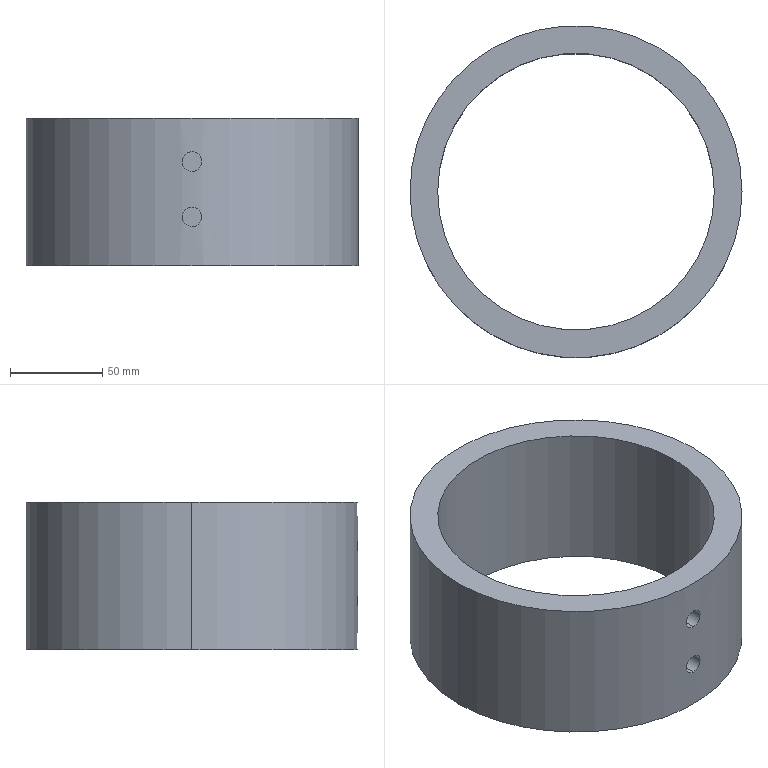Part | SolidWorks | features BaseBody 1 | 1 solid | 10 faces | box 180 x 180 x 80 mm | volume 619388 mm3 | cylinder 8 | plane 2 | commonest cylinder face diameters 10.6 x4 150 x2 180 x2
STEP:
#1=CARTESIAN_POINT('',(0.,-295.,82.3));
#2=VERTEX_POINT('',#1);
#3=CARTESIAN_POINT('',(0.,-295.,71.7));
#4=VERTEX_POINT('',#3);
#5=CARTESIAN_POINT('',(0.,-295.,82.3));
#6=CARTESIAN_POINT('',(-0.3503,-295.,82.3));
#7=CARTESIAN_POINT('',(-0.6947,-294.998,82.266));
#8=CARTESIAN_POINT('',(-1.203,-294.992,82.165));
#9=CARTESIAN_POINT('',(-1.371,-294.99,82.123));
#10=CARTESIAN_POINT('',(-1.704,-294.984,82.022));
#11=CARTESIAN_POINT('',(-1.869,-294.981,81.962));
#12=CARTESIAN_POINT('',(-2.351,-294.97,81.763));
#13=CARTESIAN_POINT('',(-2.655,-294.961,81.6));
#14=CARTESIAN_POINT('',(-3.231,-294.942,81.215));
#15=CARTESIAN_POINT('',(-3.504,-294.932,80.991));
#16=CARTESIAN_POINT('',(-3.993,-294.912,80.502));
#17=CARTESIAN_POINT('',(-4.212,-294.902,80.236));
#18=CARTESIAN_POINT('',(-4.6,-294.883,79.656));
#19=CARTESIAN_POINT('',(-4.764,-294.874,79.348));
#20=CARTESIAN_POINT('',(-5.028,-294.86,78.71));
#21=CARTESIAN_POINT('',(-5.13,-294.854,78.376));
#22=CARTESIAN_POINT('',(-5.266,-294.846,77.692));
#23=CARTESIAN_POINT('',(-5.3,-294.844,77.348));
#24=CARTESIAN_POINT('',(-5.3,-294.844,76.656));
#25=CARTESIAN_POINT('',(-5.266,-294.846,76.305));
#26=CARTESIAN_POINT('',(-5.13,-294.854,75.625));
#27=CARTESIAN_POINT('',(-5.03,-294.859,75.295));
#28=CARTESIAN_POINT('',(-4.831,-294.87,74.813));
#29=CARTESIAN_POINT('',(-4.756,-294.874,74.654));
#30=CARTESIAN_POINT('',(-4.592,-294.883,74.347));
#31=CARTESIAN_POINT('',(-4.503,-294.887,74.199));
#32=CARTESIAN_POINT('',(-4.215,-294.901,73.768));
#33=CARTESIAN_POINT('',(-3.996,-294.912,73.501));
#34=CARTESIAN_POINT('',(-3.501,-294.932,73.006));
#35=CARTESIAN_POINT('',(-3.233,-294.942,72.786));
#36=CARTESIAN_POINT('',(-2.803,-294.956,72.498));
#37=CARTESIAN_POINT('',(-2.654,-294.961,72.409));
#38=CARTESIAN_POINT('',(-2.348,-294.97,72.245));
#39=CARTESIAN_POINT('',(-2.189,-294.974,72.17));
#40=CARTESIAN_POINT('',(-1.707,-294.984,71.97));
#41=CARTESIAN_POINT('',(-1.377,-294.99,71.87));
#42=CARTESIAN_POINT('',(-0.6973,-294.998,71.735));
#43=CARTESIAN_POINT('',(-0.3459,-295.,71.7));
#44=CARTESIAN_POINT('',(0.,-295.,71.7));
#45=B_SPLINE_CURVE_WITH_KNOTS('',3,(#5,#6,#7,#8,#9,#10,#11,#12,#13,#14,#15,#16,#17,#18,#19,#20,#21,#22,#23,#24,#25,#26,#27,#28,#29,#30,#31,#32,#33,#34,#35,#36,#37,#38,#39,#40,#41,#42,#43,#44),.UNSPECIFIED.,.F.,.F.,(4,2,2,2,2,2,2,2,2,2,2,2,2,2,2,2,2,2,2,4),(0.,0.001036,0.001554,0.002072,0.003108,0.004143,0.005179,0.006215,0.007251,0.008287,0.009323,0.01036,0.01088,0.01139,0.01243,0.01347,0.01398,0.0145,0.01554,0.01657),.UNSPECIFIED.);
#46=EDGE_CURVE('',#2,#4,#45,.T.);
#47=ORIENTED_EDGE('',*,*,#46,.T.);
#48=CARTESIAN_POINT('',(0.,-280.,71.7));
#49=VERTEX_POINT('',#48);
#50=CARTESIAN_POINT('',(0.,-402.5,71.7));
#51=DIRECTION('',(0.,1.,0.));
#52=VECTOR('',#51,1000.);
#53=LINE('',#50,#52);
#54=EDGE_CURVE('',#4,#49,#53,.T.);
#55=ORIENTED_EDGE('',*,*,#54,.T.);
#56=CARTESIAN_POINT('',(0.,-280.,82.3));
#57=VERTEX_POINT('',#56);
#58=CARTESIAN_POINT('',(0.,-280.,82.3));
#59=CARTESIAN_POINT('',(-0.3503,-280.,82.3));
#60=CARTESIAN_POINT('',(-0.6947,-279.998,82.266));
#61=CARTESIAN_POINT('',(-1.203,-279.991,82.165));
#62=CARTESIAN_POINT('',(-1.371,-279.988,82.123));
#63=CARTESIAN_POINT('',(-1.704,-279.981,82.022));
#64=CARTESIAN_POINT('',(-1.869,-279.977,81.962));
#65=CARTESIAN_POINT('',(-2.351,-279.964,81.763));
#66=CARTESIAN_POINT('',(-2.655,-279.954,81.6));
#67=CARTESIAN_POINT('',(-3.231,-279.931,81.215));
#68=CARTESIAN_POINT('',(-3.504,-279.919,80.991));
#69=CARTESIAN_POINT('',(-3.993,-279.894,80.503));
#70=CARTESIAN_POINT('',(-4.212,-279.882,80.236));
#71=CARTESIAN_POINT('',(-4.6,-279.859,79.656));
#72=CARTESIAN_POINT('',(-4.764,-279.849,79.348));
#73=CARTESIAN_POINT('',(-5.028,-279.831,78.71));
#74=CARTESIAN_POINT('',(-5.13,-279.824,78.376));
#75=CARTESIAN_POINT('',(-5.266,-279.815,77.692));
#76=CARTESIAN_POINT('',(-5.3,-279.813,77.348));
#77=CARTESIAN_POINT('',(-5.3,-279.812,76.656));
#78=CARTESIAN_POINT('',(-5.266,-279.815,76.305));
#79=CARTESIAN_POINT('',(-5.13,-279.824,75.625));
#80=CARTESIAN_POINT('',(-5.03,-279.831,75.295));
#81=CARTESIAN_POINT('',(-4.831,-279.844,74.813));
#82=CARTESIAN_POINT('',(-4.756,-279.849,74.654));
#83=CARTESIAN_POINT('',(-4.592,-279.859,74.347));
#84=CARTESIAN_POINT('',(-4.503,-279.865,74.199));
#85=CARTESIAN_POINT('',(-4.215,-279.882,73.768));
#86=CARTESIAN_POINT('',(-3.996,-279.894,73.501));
#87=CARTESIAN_POINT('',(-3.501,-279.919,73.006));
#88=CARTESIAN_POINT('',(-3.233,-279.931,72.786));
#89=CARTESIAN_POINT('',(-2.803,-279.948,72.498));
#90=CARTESIAN_POINT('',(-2.654,-279.953,72.409));
#91=CARTESIAN_POINT('',(-2.348,-279.963,72.245));
#92=CARTESIAN_POINT('',(-2.189,-279.968,72.17));
#93=CARTESIAN_POINT('',(-1.707,-279.981,71.97));
#94=CARTESIAN_POINT('',(-1.377,-279.988,71.87));
#95=CARTESIAN_POINT('',(-0.6973,-279.998,71.735));
#96=CARTESIAN_POINT('',(-0.346,-280.,71.7));
#97=CARTESIAN_POINT('',(0.,-280.,71.7));
#98=B_SPLINE_CURVE_WITH_KNOTS('',3,(#58,#59,#60,#61,#62,#63,#64,#65,#66,#67,#68,#69,#70,#71,#72,#73,#74,#75,#76,#77,#78,#79,#80,#81,#82,#83,#84,#85,#86,#87,#88,#89,#90,#91,#92,#93,#94,#95,#96,#97),.UNSPECIFIED.,.F.,.F.,(4,2,2,2,2,2,2,2,2,2,2,2,2,2,2,2,2,2,2,4),(0.,0.001036,0.001554,0.002072,0.003108,0.004144,0.00518,0.006216,0.007252,0.008288,0.009324,0.01036,0.01088,0.0114,0.01243,0.01347,0.01399,0.0145,0.01554,0.01658),.UNSPECIFIED.);
#99=EDGE_CURVE('',#57,#49,#98,.T.);
#100=ORIENTED_EDGE('',*,*,#99,.F.);
#101=CARTESIAN_POINT('',(0.,-402.5,82.3));
#102=DIRECTION('',(0.,1.,0.));
#103=VECTOR('',#102,1000.);
#104=LINE('',#101,#103);
#105=EDGE_CURVE('',#2,#57,#104,.T.);
#106=ORIENTED_EDGE('',*,*,#105,.F.);
#107=EDGE_LOOP('',(#47,#55,#100,#106));
#108=FACE_OUTER_BOUND('',#107,.T.);
#109=CARTESIAN_POINT('',(0.,-402.5,77.));
#110=DIRECTION('',(0.,1.,0.));
#111=DIRECTION('',(0.,0.,1.));
#112=AXIS2_PLACEMENT_3D('',#109,#110,#111);
#113=CYLINDRICAL_SURFACE('',#112,5.3);
#114=ADVANCED_FACE('',(#108),#113,.F.);
#115=CARTESIAN_POINT('',(0.,-295.,112.3));
#116=VERTEX_POINT('',#115);
#117=CARTESIAN_POINT('',(0.,-295.,101.7));
#118=VERTEX_POINT('',#117);
#119=CARTESIAN_POINT('',(0.,-295.,112.3));
#120=CARTESIAN_POINT('',(-0.3503,-295.,112.3));
#121=CARTESIAN_POINT('',(-0.6947,-294.998,112.266));
#122=CARTESIAN_POINT('',(-1.203,-294.992,112.165));
#123=CARTESIAN_POINT('',(-1.371,-294.99,112.123));
#124=CARTESIAN_POINT('',(-1.704,-294.984,112.022));
#125=CARTESIAN_POINT('',(-1.869,-294.981,111.962));
#126=CARTESIAN_POINT('',(-2.351,-294.97,111.763));
#127=CARTESIAN_POINT('',(-2.655,-294.961,111.6));
#128=CARTESIAN_POINT('',(-3.231,-294.942,111.215));
#129=CARTESIAN_POINT('',(-3.504,-294.932,110.991));
#130=CARTESIAN_POINT('',(-3.993,-294.912,110.502));
#131=CARTESIAN_POINT('',(-4.212,-294.902,110.236));
#132=CARTESIAN_POINT('',(-4.6,-294.883,109.656));
#133=CARTESIAN_POINT('',(-4.764,-294.874,109.348));
#134=CARTESIAN_POINT('',(-5.028,-294.86,108.71));
#135=CARTESIAN_POINT('',(-5.13,-294.854,108.376));
#136=CARTESIAN_POINT('',(-5.266,-294.846,107.692));
#137=CARTESIAN_POINT('',(-5.3,-294.844,107.348));
#138=CARTESIAN_POINT('',(-5.3,-294.844,106.656));
#139=CARTESIAN_POINT('',(-5.266,-294.846,106.305));
#140=CARTESIAN_POINT('',(-5.13,-294.854,105.625));
#141=CARTESIAN_POINT('',(-5.03,-294.859,105.295));
#142=CARTESIAN_POINT('',(-4.831,-294.87,104.813));
#143=CARTESIAN_POINT('',(-4.756,-294.874,104.654));
#144=CARTESIAN_POINT('',(-4.592,-294.883,104.347));
#145=CARTESIAN_POINT('',(-4.503,-294.887,104.199));
#146=CARTESIAN_POINT('',(-4.215,-294.901,103.768));
#147=CARTESIAN_POINT('',(-3.996,-294.912,103.501));
#148=CARTESIAN_POINT('',(-3.501,-294.932,103.006));
#149=CARTESIAN_POINT('',(-3.233,-294.942,102.786));
#150=CARTESIAN_POINT('',(-2.803,-294.956,102.498));
#151=CARTESIAN_POINT('',(-2.654,-294.961,102.409));
#152=CARTESIAN_POINT('',(-2.348,-294.97,102.245));
#153=CARTESIAN_POINT('',(-2.189,-294.974,102.17));
#154=CARTESIAN_POINT('',(-1.707,-294.984,101.97));
#155=CARTESIAN_POINT('',(-1.377,-294.99,101.87));
#156=CARTESIAN_POINT('',(-0.6973,-294.998,101.735));
#157=CARTESIAN_POINT('',(-0.3459,-295.,101.7));
#158=CARTESIAN_POINT('',(0.,-295.,101.7));
#159=B_SPLINE_CURVE_WITH_KNOTS('',3,(#119,#120,#121,#122,#123,#124,#125,#126,#127,#128,#129,#130,#131,#132,#133,#134,#135,#136,#137,#138,#139,#140,#141,#142,#143,#144,#145,#146,#147,#148,#149,#150,#151,#152,#153,#154,#155,#156,#157,#158),.UNSPECIFIED.,.F.,.F.,(4,2,2,2,2,2,2,2,2,2,2,2,2,2,2,2,2,2,2,4),(0.,0.001036,0.001554,0.002072,0.003108,0.004143,0.005179,0.006215,0.007251,0.008287,0.009323,0.01036,0.01088,0.01139,0.01243,0.01347,0.01398,0.0145,0.01554,0.01657),.UNSPECIFIED.);
#160=EDGE_CURVE('',#116,#118,#159,.T.);
#161=ORIENTED_EDGE('',*,*,#160,.T.);
#162=CARTESIAN_POINT('',(0.,-280.,101.7));
#163=VERTEX_POINT('',#162);
#164=CARTESIAN_POINT('',(0.,-403.,101.7));
#165=DIRECTION('',(0.,1.,0.));
#166=VECTOR('',#165,1000.);
#167=LINE('',#164,#166);
#168=EDGE_CURVE('',#118,#163,#167,.T.);
#169=ORIENTED_EDGE('',*,*,#168,.T.);
#170=CARTESIAN_POINT('',(0.,-280.,112.3));
#171=VERTEX_POINT('',#170);
#172=CARTESIAN_POINT('',(0.,-280.,112.3));
#173=CARTESIAN_POINT('',(-0.3503,-280.,112.3));
#174=CARTESIAN_POINT('',(-0.6947,-279.998,112.266));
#175=CARTESIAN_POINT('',(-1.203,-279.991,112.165));
#176=CARTESIAN_POINT('',(-1.371,-279.988,112.123));
#177=CARTESIAN_POINT('',(-1.704,-279.981,112.022));
#178=CARTESIAN_POINT('',(-1.869,-279.977,111.962));
#179=CARTESIAN_POINT('',(-2.351,-279.964,111.763));
#180=CARTESIAN_POINT('',(-2.655,-279.954,111.6));
#181=CARTESIAN_POINT('',(-3.231,-279.931,111.215));
#182=CARTESIAN_POINT('',(-3.504,-279.919,110.991));
#183=CARTESIAN_POINT('',(-3.993,-279.894,110.503));
#184=CARTESIAN_POINT('',(-4.212,-279.882,110.236));
#185=CARTESIAN_POINT('',(-4.6,-279.859,109.656));
#186=CARTESIAN_POINT('',(-4.764,-279.849,109.348));
#187=CARTESIAN_POINT('',(-5.028,-279.831,108.71));
#188=CARTESIAN_POINT('',(-5.13,-279.824,108.376));
#189=CARTESIAN_POINT('',(-5.266,-279.815,107.692));
#190=CARTESIAN_POINT('',(-5.3,-279.813,107.348));
#191=CARTESIAN_POINT('',(-5.3,-279.812,106.656));
#192=CARTESIAN_POINT('',(-5.266,-279.815,106.305));
#193=CARTESIAN_POINT('',(-5.13,-279.824,105.625));
#194=CARTESIAN_POINT('',(-5.03,-279.831,105.295));
#195=CARTESIAN_POINT('',(-4.831,-279.844,104.813));
#196=CARTESIAN_POINT('',(-4.756,-279.849,104.654));
#197=CARTESIAN_POINT('',(-4.592,-279.859,104.347));
#198=CARTESIAN_POINT('',(-4.503,-279.865,104.199));
#199=CARTESIAN_POINT('',(-4.215,-279.882,103.768));
#200=CARTESIAN_POINT('',(-3.996,-279.894,103.501));
#201=CARTESIAN_POINT('',(-3.501,-279.919,103.006));
#202=CARTESIAN_POINT('',(-3.233,-279.931,102.786));
#203=CARTESIAN_POINT('',(-2.803,-279.948,102.498));
#204=CARTESIAN_POINT('',(-2.654,-279.953,102.409));
#205=CARTESIAN_POINT('',(-2.348,-279.963,102.245));
#206=CARTESIAN_POINT('',(-2.189,-279.968,102.17));
#207=CARTESIAN_POINT('',(-1.707,-279.981,101.97));
#208=CARTESIAN_POINT('',(-1.377,-279.988,101.87));
#209=CARTESIAN_POINT('',(-0.6973,-279.998,101.735));
#210=CARTESIAN_POINT('',(-0.346,-280.,101.7));
#211=CARTESIAN_POINT('',(0.,-280.,101.7));
#212=B_SPLINE_CURVE_WITH_KNOTS('',3,(#172,#173,#174,#175,#176,#177,#178,#179,#180,#181,#182,#183,#184,#185,#186,#187,#188,#189,#190,#191,#192,#193,#194,#195,#196,#197,#198,#199,#200,#201,#202,#203,#204,#205,#206,#207,#208,#209,#210,#211),.UNSPECIFIED.,.F.,.F.,(4,2,2,2,2,2,2,2,2,2,2,2,2,2,2,2,2,2,2,4),(0.,0.001036,0.001554,0.002072,0.003108,0.004144,0.00518,0.006216,0.007252,0.008288,0.009324,0.01036,0.01088,0.0114,0.01243,0.01347,0.01399,0.0145,0.01554,0.01658),.UNSPECIFIED.);
#213=EDGE_CURVE('',#171,#163,#212,.T.);
#214=ORIENTED_EDGE('',*,*,#213,.F.);
#215=CARTESIAN_POINT('',(0.,-403.,112.3));
#216=DIRECTION('',(0.,1.,0.));
#217=VECTOR('',#216,1000.);
#218=LINE('',#215,#217);
#219=EDGE_CURVE('',#116,#171,#218,.T.);
#220=ORIENTED_EDGE('',*,*,#219,.F.);
#221=EDGE_LOOP('',(#161,#169,#214,#220));
#222=FACE_OUTER_BOUND('',#221,.T.);
#223=CARTESIAN_POINT('',(0.,-403.,107.));
#224=DIRECTION('',(0.,1.,0.));
#225=DIRECTION('',(0.,0.,1.));
#226=AXIS2_PLACEMENT_3D('',#223,#224,#225);
#227=CYLINDRICAL_SURFACE('',#226,5.3);
#228=ADVANCED_FACE('',(#222),#227,.F.);
#229=ORIENTED_EDGE('',*,*,#99,.T.);
#230=CARTESIAN_POINT('',(0.,-280.,71.7));
#231=CARTESIAN_POINT('',(0.3459,-280.,71.7));
#232=CARTESIAN_POINT('',(0.6897,-279.998,71.734));
#233=CARTESIAN_POINT('',(1.202,-279.991,71.835));
#234=CARTESIAN_POINT('',(1.373,-279.988,71.878));
#235=CARTESIAN_POINT('',(1.705,-279.981,71.979));
#236=CARTESIAN_POINT('',(1.867,-279.977,72.037));
#237=CARTESIAN_POINT('',(2.346,-279.964,72.235));
#238=CARTESIAN_POINT('',(2.654,-279.954,72.399));
#239=CARTESIAN_POINT('',(3.234,-279.931,72.786));
#240=CARTESIAN_POINT('',(3.501,-279.919,73.006));
#241=CARTESIAN_POINT('',(3.99,-279.894,73.494));
#242=CARTESIAN_POINT('',(4.213,-279.882,73.766));
#243=CARTESIAN_POINT('',(4.599,-279.859,74.342));
#244=CARTESIAN_POINT('',(4.761,-279.849,74.646));
#245=CARTESIAN_POINT('',(4.961,-279.836,75.127));
#246=CARTESIAN_POINT('',(5.02,-279.832,75.293));
#247=CARTESIAN_POINT('',(5.122,-279.825,75.626));
#248=CARTESIAN_POINT('',(5.164,-279.822,75.794));
#249=CARTESIAN_POINT('',(5.265,-279.815,76.302));
#250=CARTESIAN_POINT('',(5.3,-279.813,76.646));
#251=CARTESIAN_POINT('',(5.3,-279.812,77.346));
#252=CARTESIAN_POINT('',(5.266,-279.815,77.691));
#253=CARTESIAN_POINT('',(5.165,-279.822,78.199));
#254=CARTESIAN_POINT('',(5.124,-279.825,78.367));
#255=CARTESIAN_POINT('',(5.023,-279.832,78.7));
#256=CARTESIAN_POINT('',(4.964,-279.836,78.865));
#257=CARTESIAN_POINT('',(4.765,-279.849,79.347));
#258=CARTESIAN_POINT('',(4.602,-279.859,79.652));
#259=CARTESIAN_POINT('',(4.218,-279.882,80.227));
#260=CARTESIAN_POINT('',(3.995,-279.894,80.5));
#261=CARTESIAN_POINT('',(3.506,-279.918,80.99));
#262=CARTESIAN_POINT('',(3.24,-279.931,81.209));
#263=CARTESIAN_POINT('',(2.806,-279.948,81.5));
#264=CARTESIAN_POINT('',(2.655,-279.953,81.59));
#265=CARTESIAN_POINT('',(2.349,-279.963,81.754));
#266=CARTESIAN_POINT('',(2.193,-279.968,81.828));
#267=CARTESIAN_POINT('',(1.715,-279.981,82.027));
#268=CARTESIAN_POINT('',(1.382,-279.988,82.129));
#269=CARTESIAN_POINT('',(0.6967,-279.998,82.266));
#270=CARTESIAN_POINT('',(0.3502,-280.,82.3));
#271=CARTESIAN_POINT('',(0.,-280.,82.3));
#272=B_SPLINE_CURVE_WITH_KNOTS('',3,(#230,#231,#232,#233,#234,#235,#236,#237,#238,#239,#240,#241,#242,#243,#244,#245,#246,#247,#248,#249,#250,#251,#252,#253,#254,#255,#256,#257,#258,#259,#260,#261,#262,#263,#264,#265,#266,#267,#268,#269,#270,#271),.UNSPECIFIED.,.F.,.F.,(4,2,2,2,2,2,2,2,2,2,2,2,2,2,2,2,2,2,2,2,4),(0.01658,0.01761,0.01813,0.01865,0.01968,0.02072,0.02175,0.02279,0.02331,0.02383,0.02486,0.0259,0.02641,0.02693,0.02797,0.029,0.03004,0.03056,0.03108,0.03211,0.03315),.UNSPECIFIED.);
#273=EDGE_CURVE('',#49,#57,#272,.T.);
#274=ORIENTED_EDGE('',*,*,#273,.T.);
#275=EDGE_LOOP('',(#229,#274));
#276=FACE_BOUND('',#275,.T.);
#277=ORIENTED_EDGE('',*,*,#213,.T.);
#278=CARTESIAN_POINT('',(0.,-280.,101.7));
#279=CARTESIAN_POINT('',(0.3459,-280.,101.7));
#280=CARTESIAN_POINT('',(0.6897,-279.998,101.734));
#281=CARTESIAN_POINT('',(1.202,-279.991,101.835));
#282=CARTESIAN_POINT('',(1.373,-279.988,101.878));
#283=CARTESIAN_POINT('',(1.705,-279.981,101.979));
#284=CARTESIAN_POINT('',(1.867,-279.977,102.037));
#285=CARTESIAN_POINT('',(2.346,-279.964,102.235));
#286=CARTESIAN_POINT('',(2.654,-279.954,102.399));
#287=CARTESIAN_POINT('',(3.234,-279.931,102.786));
#288=CARTESIAN_POINT('',(3.501,-279.919,103.006));
#289=CARTESIAN_POINT('',(3.99,-279.894,103.494));
#290=CARTESIAN_POINT('',(4.213,-279.882,103.766));
#291=CARTESIAN_POINT('',(4.599,-279.859,104.342));
#292=CARTESIAN_POINT('',(4.761,-279.849,104.646));
#293=CARTESIAN_POINT('',(4.961,-279.836,105.127));
#294=CARTESIAN_POINT('',(5.02,-279.832,105.293));
#295=CARTESIAN_POINT('',(5.122,-279.825,105.626));
#296=CARTESIAN_POINT('',(5.164,-279.822,105.794));
#297=CARTESIAN_POINT('',(5.265,-279.815,106.302));
#298=CARTESIAN_POINT('',(5.3,-279.813,106.646));
#299=CARTESIAN_POINT('',(5.3,-279.812,107.346));
#300=CARTESIAN_POINT('',(5.266,-279.815,107.691));
#301=CARTESIAN_POINT('',(5.165,-279.822,108.199));
#302=CARTESIAN_POINT('',(5.124,-279.825,108.367));
#303=CARTESIAN_POINT('',(5.023,-279.832,108.7));
#304=CARTESIAN_POINT('',(4.964,-279.836,108.865));
#305=CARTESIAN_POINT('',(4.765,-279.849,109.347));
#306=CARTESIAN_POINT('',(4.602,-279.859,109.652));
#307=CARTESIAN_POINT('',(4.218,-279.882,110.227));
#308=CARTESIAN_POINT('',(3.995,-279.894,110.5));
#309=CARTESIAN_POINT('',(3.506,-279.918,110.99));
#310=CARTESIAN_POINT('',(3.24,-279.931,111.209));
#311=CARTESIAN_POINT('',(2.806,-279.948,111.5));
#312=CARTESIAN_POINT('',(2.655,-279.953,111.59));
#313=CARTESIAN_POINT('',(2.349,-279.963,111.754));
#314=CARTESIAN_POINT('',(2.193,-279.968,111.828));
#315=CARTESIAN_POINT('',(1.715,-279.981,112.027));
#316=CARTESIAN_POINT('',(1.382,-279.988,112.129));
#317=CARTESIAN_POINT('',(0.6967,-279.998,112.266));
#318=CARTESIAN_POINT('',(0.3502,-280.,112.3));
#319=CARTESIAN_POINT('',(0.,-280.,112.3));
#320=B_SPLINE_CURVE_WITH_KNOTS('',3,(#278,#279,#280,#281,#282,#283,#284,#285,#286,#287,#288,#289,#290,#291,#292,#293,#294,#295,#296,#297,#298,#299,#300,#301,#302,#303,#304,#305,#306,#307,#308,#309,#310,#311,#312,#313,#314,#315,#316,#317,#318,#319),.UNSPECIFIED.,.F.,.F.,(4,2,2,2,2,2,2,2,2,2,2,2,2,2,2,2,2,2,2,2,4),(0.01658,0.01761,0.01813,0.01865,0.01968,0.02072,0.02175,0.02279,0.02331,0.02383,0.02486,0.0259,0.02641,0.02693,0.02797,0.029,0.03004,0.03056,0.03108,0.03211,0.03315),.UNSPECIFIED.);
#321=EDGE_CURVE('',#163,#171,#320,.T.);
#322=ORIENTED_EDGE('',*,*,#321,.T.);
#323=EDGE_LOOP('',(#277,#322));
#324=FACE_BOUND('',#323,.T.);
#325=CARTESIAN_POINT('',(-75.,-205.,130.5));
#326=VERTEX_POINT('',#325);
#327=CARTESIAN_POINT('',(75.,-205.,130.5));
#328=VERTEX_POINT('',#327);
#329=CARTESIAN_POINT('',(0.,-205.,130.5));
#330=DIRECTION('',(0.,0.,1.));
#331=DIRECTION('',(1.,0.,0.));
#332=AXIS2_PLACEMENT_3D('',#329,#330,#331);
#333=CIRCLE('',#332,75.);
#334=EDGE_CURVE('',#326,#328,#333,.T.);
#335=ORIENTED_EDGE('',*,*,#334,.T.);
#336=CARTESIAN_POINT('',(75.,-205.,50.5));
#337=VERTEX_POINT('',#336);
#338=CARTESIAN_POINT('',(75.,-205.,170.5));
#339=DIRECTION('',(0.,0.,-1.));
#340=VECTOR('',#339,1000.);
#341=LINE('',#338,#340);
#342=EDGE_CURVE('',#328,#337,#341,.T.);
#343=ORIENTED_EDGE('',*,*,#342,.T.);
#344=CARTESIAN_POINT('',(-75.,-205.,50.5));
#345=VERTEX_POINT('',#344);
#346=CARTESIAN_POINT('',(0.,-205.,50.5));
#347=DIRECTION('',(0.,0.,-1.));
#348=DIRECTION('',(-1.,0.,0.));
#349=AXIS2_PLACEMENT_3D('',#346,#347,#348);
#350=CIRCLE('',#349,75.);
#351=EDGE_CURVE('',#337,#345,#350,.T.);
#352=ORIENTED_EDGE('',*,*,#351,.T.);
#353=CARTESIAN_POINT('',(-75.,-205.,170.5));
#354=DIRECTION('',(0.,0.,-1.));
#355=VECTOR('',#354,1000.);
#356=LINE('',#353,#355);
#357=EDGE_CURVE('',#326,#345,#356,.T.);
#358=ORIENTED_EDGE('',*,*,#357,.F.);
#359=EDGE_LOOP('',(#335,#343,#352,#358));
#360=FACE_OUTER_BOUND('',#359,.T.);
#361=CARTESIAN_POINT('',(0.,-205.,170.5));
#362=DIRECTION('',(0.,0.,-1.));
#363=DIRECTION('',(-1.,0.,0.));
#364=AXIS2_PLACEMENT_3D('',#361,#362,#363);
#365=CYLINDRICAL_SURFACE('',#364,75.);
#366=ADVANCED_FACE('',(#276,#324,#360),#365,.F.);
#367=CARTESIAN_POINT('',(-90.,-205.,130.5));
#368=VERTEX_POINT('',#367);
#369=CARTESIAN_POINT('',(90.,-205.,130.5));
#370=VERTEX_POINT('',#369);
#371=CARTESIAN_POINT('',(0.,-205.,130.5));
#372=DIRECTION('',(0.,0.,-1.));
#373=DIRECTION('',(-1.,0.,0.));
#374=AXIS2_PLACEMENT_3D('',#371,#372,#373);
#375=CIRCLE('',#374,90.);
#376=EDGE_CURVE('',#368,#370,#375,.T.);
#377=ORIENTED_EDGE('',*,*,#376,.T.);
#378=CARTESIAN_POINT('',(90.,-205.,50.5));
#379=VERTEX_POINT('',#378);
#380=CARTESIAN_POINT('',(90.,-205.,130.5));
#381=DIRECTION('',(0.,0.,-1.));
#382=VECTOR('',#381,1000.);
#383=LINE('',#380,#382);
#384=EDGE_CURVE('',#370,#379,#383,.T.);
#385=ORIENTED_EDGE('',*,*,#384,.T.);
#386=CARTESIAN_POINT('',(-90.,-205.,50.5));
#387=VERTEX_POINT('',#386);
#388=CARTESIAN_POINT('',(0.,-205.,50.5));
#389=DIRECTION('',(0.,0.,-1.));
#390=DIRECTION('',(-1.,0.,0.));
#391=AXIS2_PLACEMENT_3D('',#388,#389,#390);
#392=CIRCLE('',#391,90.);
#393=EDGE_CURVE('',#387,#379,#392,.T.);
#394=ORIENTED_EDGE('',*,*,#393,.F.);
#395=CARTESIAN_POINT('',(-90.,-205.,130.5));
#396=DIRECTION('',(0.,0.,-1.));
#397=VECTOR('',#396,1000.);
#398=LINE('',#395,#397);
#399=EDGE_CURVE('',#368,#387,#398,.T.);
#400=ORIENTED_EDGE('',*,*,#399,.F.);
#401=EDGE_LOOP('',(#377,#385,#394,#400));
#402=FACE_OUTER_BOUND('',#401,.T.);
#403=CARTESIAN_POINT('',(0.,-205.,130.5));
#404=DIRECTION('',(0.,0.,-1.));
#405=DIRECTION('',(-1.,0.,0.));
#406=AXIS2_PLACEMENT_3D('',#403,#404,#405);
#407=CYLINDRICAL_SURFACE('',#406,90.);
#408=ADVANCED_FACE('',(#402),#407,.T.);
#409=ORIENTED_EDGE('',*,*,#384,.F.);
#410=CARTESIAN_POINT('',(0.,-205.,130.5));
#411=DIRECTION('',(0.,0.,-1.));
#412=DIRECTION('',(-1.,0.,0.));
#413=AXIS2_PLACEMENT_3D('',#410,#411,#412);
#414=CIRCLE('',#413,90.);
#415=EDGE_CURVE('',#370,#368,#414,.T.);
#416=ORIENTED_EDGE('',*,*,#415,.T.);
#417=ORIENTED_EDGE('',*,*,#399,.T.);
#418=CARTESIAN_POINT('',(0.,-205.,50.5));
#419=DIRECTION('',(0.,0.,-1.));
#420=DIRECTION('',(-1.,0.,0.));
#421=AXIS2_PLACEMENT_3D('',#418,#419,#420);
#422=CIRCLE('',#421,90.);
#423=EDGE_CURVE('',#379,#387,#422,.T.);
#424=ORIENTED_EDGE('',*,*,#423,.F.);
#425=EDGE_LOOP('',(#409,#416,#417,#424));
#426=FACE_OUTER_BOUND('',#425,.T.);
#427=ORIENTED_EDGE('',*,*,#46,.F.);
#428=CARTESIAN_POINT('',(0.,-295.,71.7));
#429=CARTESIAN_POINT('',(0.3459,-295.,71.7));
#430=CARTESIAN_POINT('',(0.6897,-294.998,71.734));
#431=CARTESIAN_POINT('',(1.202,-294.992,71.835));
#432=CARTESIAN_POINT('',(1.373,-294.99,71.878));
#433=CARTESIAN_POINT('',(1.705,-294.984,71.979));
#434=CARTESIAN_POINT('',(1.867,-294.981,72.037));
#435=CARTESIAN_POINT('',(2.346,-294.97,72.235));
#436=CARTESIAN_POINT('',(2.653,-294.961,72.399));
#437=CARTESIAN_POINT('',(3.234,-294.942,72.786));
#438=CARTESIAN_POINT('',(3.501,-294.932,73.006));
#439=CARTESIAN_POINT('',(3.99,-294.912,73.494));
#440=CARTESIAN_POINT('',(4.213,-294.902,73.766));
#441=CARTESIAN_POINT('',(4.599,-294.883,74.342));
#442=CARTESIAN_POINT('',(4.761,-294.874,74.647));
#443=CARTESIAN_POINT('',(4.961,-294.863,75.127));
#444=CARTESIAN_POINT('',(5.02,-294.86,75.293));
#445=CARTESIAN_POINT('',(5.122,-294.854,75.626));
#446=CARTESIAN_POINT('',(5.164,-294.852,75.794));
#447=CARTESIAN_POINT('',(5.265,-294.846,76.302));
#448=CARTESIAN_POINT('',(5.3,-294.844,76.646));
#449=CARTESIAN_POINT('',(5.3,-294.844,77.345));
#450=CARTESIAN_POINT('',(5.266,-294.846,77.691));
#451=CARTESIAN_POINT('',(5.166,-294.852,78.199));
#452=CARTESIAN_POINT('',(5.124,-294.854,78.367));
#453=CARTESIAN_POINT('',(5.023,-294.86,78.699));
#454=CARTESIAN_POINT('',(4.964,-294.863,78.865));
#455=CARTESIAN_POINT('',(4.765,-294.874,79.347));
#456=CARTESIAN_POINT('',(4.602,-294.882,79.651));
#457=CARTESIAN_POINT('',(4.218,-294.901,80.227));
#458=CARTESIAN_POINT('',(3.995,-294.912,80.5));
#459=CARTESIAN_POINT('',(3.506,-294.932,80.99));
#460=CARTESIAN_POINT('',(3.239,-294.942,81.209));
#461=CARTESIAN_POINT('',(2.806,-294.956,81.5));
#462=CARTESIAN_POINT('',(2.655,-294.961,81.59));
#463=CARTESIAN_POINT('',(2.349,-294.969,81.754));
#464=CARTESIAN_POINT('',(2.193,-294.973,81.828));
#465=CARTESIAN_POINT('',(1.715,-294.984,82.027));
#466=CARTESIAN_POINT('',(1.382,-294.99,82.129));
#467=CARTESIAN_POINT('',(0.6967,-294.998,82.266));
#468=CARTESIAN_POINT('',(0.3502,-295.,82.3));
#469=CARTESIAN_POINT('',(0.,-295.,82.3));
#470=B_SPLINE_CURVE_WITH_KNOTS('',3,(#428,#429,#430,#431,#432,#433,#434,#435,#436,#437,#438,#439,#440,#441,#442,#443,#444,#445,#446,#447,#448,#449,#450,#451,#452,#453,#454,#455,#456,#457,#458,#459,#460,#461,#462,#463,#464,#465,#466,#467,#468,#469),.UNSPECIFIED.,.F.,.F.,(4,2,2,2,2,2,2,2,2,2,2,2,2,2,2,2,2,2,2,2,4),(0.01657,0.01761,0.01813,0.01865,0.01968,0.02072,0.02175,0.02279,0.02331,0.02382,0.02486,0.02589,0.02641,0.02693,0.02797,0.029,0.03004,0.03055,0.03107,0.03211,0.03314),.UNSPECIFIED.);
#471=EDGE_CURVE('',#4,#2,#470,.T.);
#472=ORIENTED_EDGE('',*,*,#471,.F.);
#473=EDGE_LOOP('',(#427,#472));
#474=FACE_BOUND('',#473,.T.);
#475=ORIENTED_EDGE('',*,*,#160,.F.);
#476=CARTESIAN_POINT('',(0.,-295.,101.7));
#477=CARTESIAN_POINT('',(0.3459,-295.,101.7));
#478=CARTESIAN_POINT('',(0.6897,-294.998,101.734));
#479=CARTESIAN_POINT('',(1.202,-294.992,101.835));
#480=CARTESIAN_POINT('',(1.373,-294.99,101.878));
#481=CARTESIAN_POINT('',(1.705,-294.984,101.979));
#482=CARTESIAN_POINT('',(1.867,-294.981,102.037));
#483=CARTESIAN_POINT('',(2.346,-294.97,102.235));
#484=CARTESIAN_POINT('',(2.653,-294.961,102.399));
#485=CARTESIAN_POINT('',(3.234,-294.942,102.786));
#486=CARTESIAN_POINT('',(3.501,-294.932,103.006));
#487=CARTESIAN_POINT('',(3.99,-294.912,103.494));
#488=CARTESIAN_POINT('',(4.213,-294.902,103.766));
#489=CARTESIAN_POINT('',(4.599,-294.883,104.342));
#490=CARTESIAN_POINT('',(4.761,-294.874,104.647));
#491=CARTESIAN_POINT('',(4.961,-294.863,105.127));
#492=CARTESIAN_POINT('',(5.02,-294.86,105.293));
#493=CARTESIAN_POINT('',(5.122,-294.854,105.626));
#494=CARTESIAN_POINT('',(5.164,-294.852,105.794));
#495=CARTESIAN_POINT('',(5.265,-294.846,106.302));
#496=CARTESIAN_POINT('',(5.3,-294.844,106.646));
#497=CARTESIAN_POINT('',(5.3,-294.844,107.345));
#498=CARTESIAN_POINT('',(5.266,-294.846,107.691));
#499=CARTESIAN_POINT('',(5.166,-294.852,108.199));
#500=CARTESIAN_POINT('',(5.124,-294.854,108.367));
#501=CARTESIAN_POINT('',(5.023,-294.86,108.699));
#502=CARTESIAN_POINT('',(4.964,-294.863,108.865));
#503=CARTESIAN_POINT('',(4.765,-294.874,109.347));
#504=CARTESIAN_POINT('',(4.602,-294.882,109.651));
#505=CARTESIAN_POINT('',(4.218,-294.901,110.227));
#506=CARTESIAN_POINT('',(3.995,-294.912,110.5));
#507=CARTESIAN_POINT('',(3.506,-294.932,110.99));
#508=CARTESIAN_POINT('',(3.239,-294.942,111.209));
#509=CARTESIAN_POINT('',(2.806,-294.956,111.5));
#510=CARTESIAN_POINT('',(2.655,-294.961,111.59));
#511=CARTESIAN_POINT('',(2.349,-294.969,111.754));
#512=CARTESIAN_POINT('',(2.193,-294.973,111.828));
#513=CARTESIAN_POINT('',(1.715,-294.984,112.027));
#514=CARTESIAN_POINT('',(1.382,-294.99,112.129));
#515=CARTESIAN_POINT('',(0.6967,-294.998,112.266));
#516=CARTESIAN_POINT('',(0.3502,-295.,112.3));
#517=CARTESIAN_POINT('',(0.,-295.,112.3));
#518=B_SPLINE_CURVE_WITH_KNOTS('',3,(#476,#477,#478,#479,#480,#481,#482,#483,#484,#485,#486,#487,#488,#489,#490,#491,#492,#493,#494,#495,#496,#497,#498,#499,#500,#501,#502,#503,#504,#505,#506,#507,#508,#509,#510,#511,#512,#513,#514,#515,#516,#517),.UNSPECIFIED.,.F.,.F.,(4,2,2,2,2,2,2,2,2,2,2,2,2,2,2,2,2,2,2,2,4),(0.01657,0.01761,0.01813,0.01865,0.01968,0.02072,0.02175,0.02279,0.02331,0.02382,0.02486,0.02589,0.02641,0.02693,0.02797,0.029,0.03004,0.03055,0.03107,0.03211,0.03314),.UNSPECIFIED.);
#519=EDGE_CURVE('',#118,#116,#518,.T.);
#520=ORIENTED_EDGE('',*,*,#519,.F.);
#521=EDGE_LOOP('',(#475,#520));
#522=FACE_BOUND('',#521,.T.);
#523=CARTESIAN_POINT('',(0.,-205.,130.5));
#524=DIRECTION('',(0.,0.,-1.));
#525=DIRECTION('',(-1.,0.,0.));
#526=AXIS2_PLACEMENT_3D('',#523,#524,#525);
#527=CYLINDRICAL_SURFACE('',#526,90.);
#528=ADVANCED_FACE('',(#426,#474,#522),#527,.T.);
#529=ORIENTED_EDGE('',*,*,#342,.F.);
#530=CARTESIAN_POINT('',(0.,-205.,130.5));
#531=DIRECTION('',(0.,0.,1.));
#532=DIRECTION('',(1.,0.,0.));
#533=AXIS2_PLACEMENT_3D('',#530,#531,#532);
#534=CIRCLE('',#533,75.);
#535=EDGE_CURVE('',#328,#326,#534,.T.);
#536=ORIENTED_EDGE('',*,*,#535,.T.);
#537=ORIENTED_EDGE('',*,*,#357,.T.);
#538=CARTESIAN_POINT('',(0.,-205.,50.5));
#539=DIRECTION('',(0.,0.,-1.));
#540=DIRECTION('',(-1.,0.,0.));
#541=AXIS2_PLACEMENT_3D('',#538,#539,#540);
#542=CIRCLE('',#541,75.);
#543=EDGE_CURVE('',#345,#337,#542,.T.);
#544=ORIENTED_EDGE('',*,*,#543,.T.);
#545=EDGE_LOOP('',(#529,#536,#537,#544));
#546=FACE_OUTER_BOUND('',#545,.T.);
#547=CARTESIAN_POINT('',(0.,-205.,170.5));
#548=DIRECTION('',(0.,0.,-1.));
#549=DIRECTION('',(-1.,0.,0.));
#550=AXIS2_PLACEMENT_3D('',#547,#548,#549);
#551=CYLINDRICAL_SURFACE('',#550,75.);
#552=ADVANCED_FACE('',(#546),#551,.F.);
#553=ORIENTED_EDGE('',*,*,#543,.F.);
#554=ORIENTED_EDGE('',*,*,#351,.F.);
#555=EDGE_LOOP('',(#553,#554));
#556=FACE_BOUND('',#555,.T.);
#557=ORIENTED_EDGE('',*,*,#393,.T.);
#558=ORIENTED_EDGE('',*,*,#423,.T.);
#559=EDGE_LOOP('',(#557,#558));
#560=FACE_OUTER_BOUND('',#559,.T.);
#561=CARTESIAN_POINT('',(0.,-205.,50.5));
#562=DIRECTION('',(0.,0.,-1.));
#563=DIRECTION('',(-1.,0.,0.));
#564=AXIS2_PLACEMENT_3D('',#561,#562,#563);
#565=PLANE('',#564);
#566=ADVANCED_FACE('',(#556,#560),#565,.T.);
#567=ORIENTED_EDGE('',*,*,#334,.F.);
#568=ORIENTED_EDGE('',*,*,#535,.F.);
#569=EDGE_LOOP('',(#567,#568));
#570=FACE_BOUND('',#569,.T.);
#571=ORIENTED_EDGE('',*,*,#376,.F.);
#572=ORIENTED_EDGE('',*,*,#415,.F.);
#573=EDGE_LOOP('',(#571,#572));
#574=FACE_OUTER_BOUND('',#573,.T.);
#575=CARTESIAN_POINT('',(0.,-205.,130.5));
#576=DIRECTION('',(0.,0.,1.));
#577=DIRECTION('',(1.,0.,0.));
#578=AXIS2_PLACEMENT_3D('',#575,#576,#577);
#579=PLANE('',#578);
#580=ADVANCED_FACE('',(#570,#574),#579,.T.);
#581=ORIENTED_EDGE('',*,*,#168,.F.);
#582=ORIENTED_EDGE('',*,*,#519,.T.);
#583=ORIENTED_EDGE('',*,*,#219,.T.);
#584=ORIENTED_EDGE('',*,*,#321,.F.);
#585=EDGE_LOOP('',(#581,#582,#583,#584));
#586=FACE_OUTER_BOUND('',#585,.T.);
#587=CARTESIAN_POINT('',(0.,-403.,107.));
#588=DIRECTION('',(0.,1.,0.));
#589=DIRECTION('',(0.,0.,1.));
#590=AXIS2_PLACEMENT_3D('',#587,#588,#589);
#591=CYLINDRICAL_SURFACE('',#590,5.3);
#592=ADVANCED_FACE('',(#586),#591,.F.);
#593=ORIENTED_EDGE('',*,*,#54,.F.);
#594=ORIENTED_EDGE('',*,*,#471,.T.);
#595=ORIENTED_EDGE('',*,*,#105,.T.);
#596=ORIENTED_EDGE('',*,*,#273,.F.);
#597=EDGE_LOOP('',(#593,#594,#595,#596));
#598=FACE_OUTER_BOUND('',#597,.T.);
#599=CARTESIAN_POINT('',(0.,-402.5,77.));
#600=DIRECTION('',(0.,1.,0.));
#601=DIRECTION('',(0.,0.,1.));
#602=AXIS2_PLACEMENT_3D('',#599,#600,#601);
#603=CYLINDRICAL_SURFACE('',#602,5.3);
#604=ADVANCED_FACE('',(#598),#603,.F.);
#605=CLOSED_SHELL('',(#114,#228,#366,#408,#528,#552,#566,#580,#592,#604));
#606=MANIFOLD_SOLID_BREP('',#605);
#607=CARTESIAN_POINT('',(0.,0.,0.));
#608=DIRECTION('',(0.,0.,1.));
#609=DIRECTION('',(1.,0.,0.));
#610=AXIS2_PLACEMENT_3D('',#607,#608,#609);
#611=(LENGTH_UNIT()NAMED_UNIT(*)SI_UNIT(.MILLI.,.METRE.));
#612=UNCERTAINTY_MEASURE_WITH_UNIT(LENGTH_MEASURE(0.00001),#611,'','');
#613=(NAMED_UNIT(*)PLANE_ANGLE_UNIT()SI_UNIT($,.RADIAN.));
#614=(NAMED_UNIT(*)SI_UNIT($,.STERADIAN.)SOLID_ANGLE_UNIT());
#615=(GEOMETRIC_REPRESENTATION_CONTEXT(3)GLOBAL_UNCERTAINTY_ASSIGNED_CONTEXT((#612))GLOBAL_UNIT_ASSIGNED_CONTEXT((#611,#613,#614))REPRESENTATION_CONTEXT('',''));
#616=ADVANCED_BREP_SHAPE_REPRESENTATION('',(#606,#610),#615);